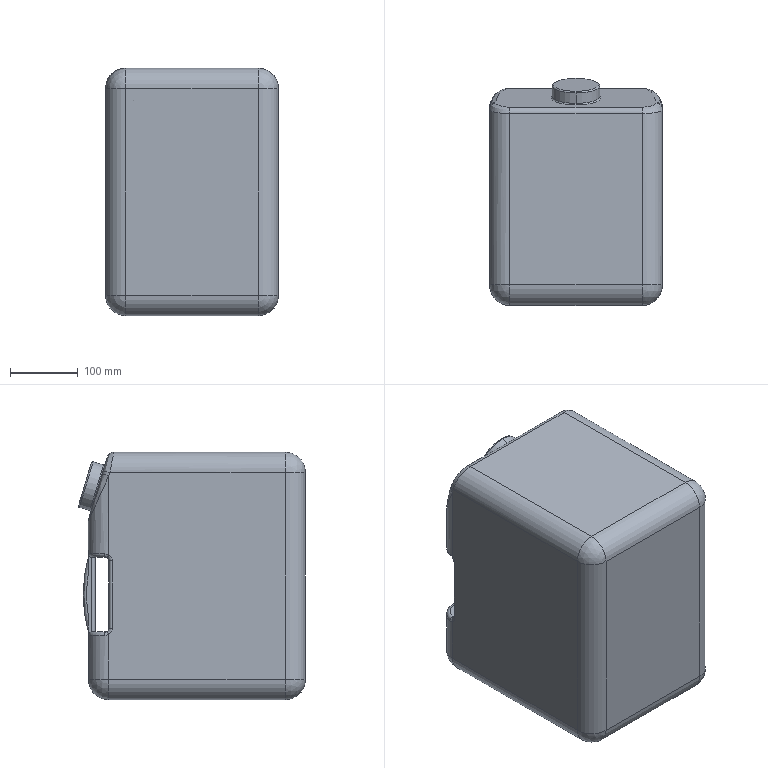Part | 1 solid | 73 faces | box 255 x 334.589 x 365 mm | volume 28104400 mm3 | cylinder 30 | plane 15 | torus 14 | spline 8 | sphere 6 | commonest cylinder face diameters 60 x13 10 x10 20 x4 70 x2 400 x1